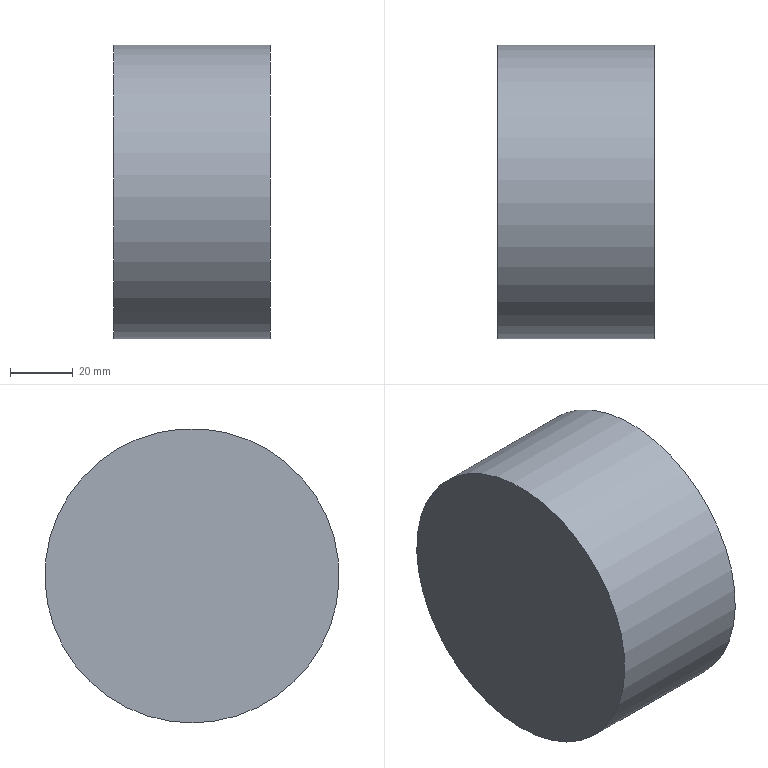Part | NX | features solid 2 | 1 solid | 3 faces | box 50 x 94.142 x 94.142 mm | volume 348039 mm3 | plane 2 | cylinder 1 | commonest cylinder face diameters 94.142 x1
STEP:
#1=CARTESIAN_POINT('',(1075.,230.,-217.071));
#2=VERTEX_POINT('',#1);
#3=CARTESIAN_POINT('',(1075.,230.,-170.));
#4=DIRECTION('',(-1.,0.,0.));
#5=DIRECTION('',(0.,0.,-1.));
#6=AXIS2_PLACEMENT_3D('',#3,#4,#5);
#7=CIRCLE('',#6,47.071);
#8=EDGE_CURVE('',#2,#2,#7,.T.);
#9=ORIENTED_EDGE('',*,*,#8,.F.);
#10=EDGE_LOOP('',(#9));
#11=FACE_BOUND('',#10,.T.);
#12=CARTESIAN_POINT('',(1125.,230.,-217.071));
#13=VERTEX_POINT('',#12);
#14=CARTESIAN_POINT('',(1125.,230.,-170.));
#15=DIRECTION('',(-1.,0.,0.));
#16=DIRECTION('',(0.,0.,-1.));
#17=AXIS2_PLACEMENT_3D('',#14,#15,#16);
#18=CIRCLE('',#17,47.071);
#19=EDGE_CURVE('',#13,#13,#18,.T.);
#20=ORIENTED_EDGE('',*,*,#19,.T.);
#21=EDGE_LOOP('',(#20));
#22=FACE_BOUND('',#21,.T.);
#23=CARTESIAN_POINT('',(1075.,230.,-170.));
#24=DIRECTION('',(1.,0.,0.));
#25=DIRECTION('',(0.,0.,-1.));
#26=AXIS2_PLACEMENT_3D('',#23,#24,#25);
#27=CYLINDRICAL_SURFACE('',#26,47.071);
#28=ADVANCED_FACE('',(#11,#22),#27,.T.);
#29=ORIENTED_EDGE('',*,*,#8,.T.);
#30=EDGE_LOOP('',(#29));
#31=FACE_BOUND('',#30,.T.);
#32=CARTESIAN_POINT('',(1075.,230.,-170.));
#33=DIRECTION('',(-1.,0.,0.));
#34=DIRECTION('',(0.,0.,-1.));
#35=AXIS2_PLACEMENT_3D('',#32,#33,#34);
#36=PLANE('',#35);
#37=ADVANCED_FACE('',(#31),#36,.T.);
#38=ORIENTED_EDGE('',*,*,#19,.F.);
#39=EDGE_LOOP('',(#38));
#40=FACE_BOUND('',#39,.T.);
#41=CARTESIAN_POINT('',(1125.,230.,-170.));
#42=DIRECTION('',(-1.,0.,0.));
#43=DIRECTION('',(0.,0.,-1.));
#44=AXIS2_PLACEMENT_3D('',#41,#42,#43);
#45=PLANE('',#44);
#46=ADVANCED_FACE('',(#40),#45,.F.);
#47=CLOSED_SHELL('',(#28,#37,#46));
#48=MANIFOLD_SOLID_BREP('',#47);
#49=(LENGTH_UNIT()NAMED_UNIT(*)SI_UNIT(.MILLI.,.METRE.));
#50=UNCERTAINTY_MEASURE_WITH_UNIT(LENGTH_MEASURE(0.00001),#49,'','');
#51=(NAMED_UNIT(*)PLANE_ANGLE_UNIT()SI_UNIT($,.RADIAN.));
#52=(NAMED_UNIT(*)SI_UNIT($,.STERADIAN.)SOLID_ANGLE_UNIT());
#53=(GEOMETRIC_REPRESENTATION_CONTEXT(3)GLOBAL_UNCERTAINTY_ASSIGNED_CONTEXT((#50))GLOBAL_UNIT_ASSIGNED_CONTEXT((#49,#51,#52))REPRESENTATION_CONTEXT('',''));
#54=ADVANCED_BREP_SHAPE_REPRESENTATION('',(#48),#53);